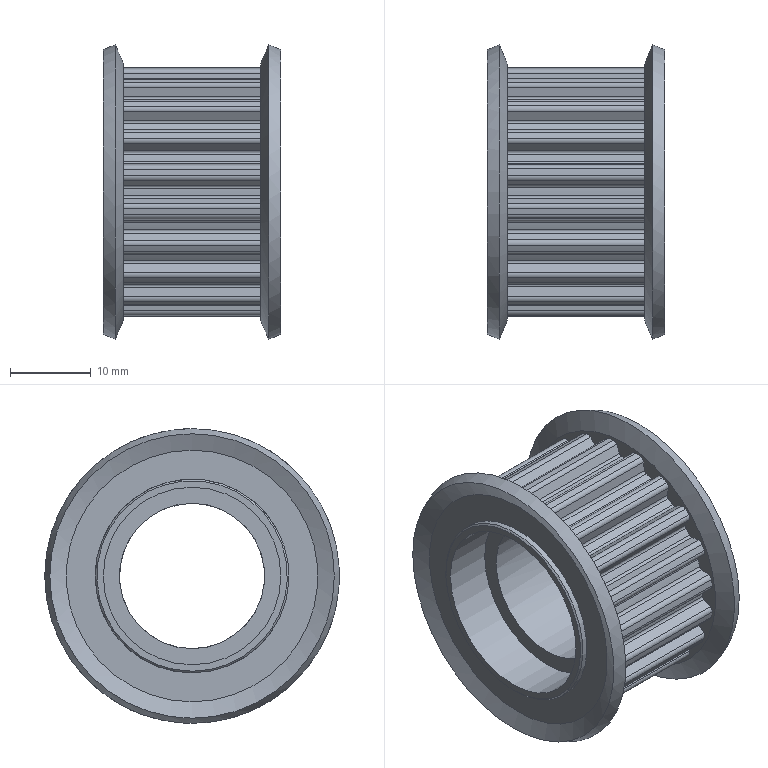Part | NX | 1 solid | 180 faces | box 22 x 36.509 x 36.509 mm | volume 8405 mm3 | cylinder 125 | plane 48 | cone 7 | commonest cylinder face diameters 0.8 x40 1.2 x40 27.4 x20 31 x20 22 x2 24 x2